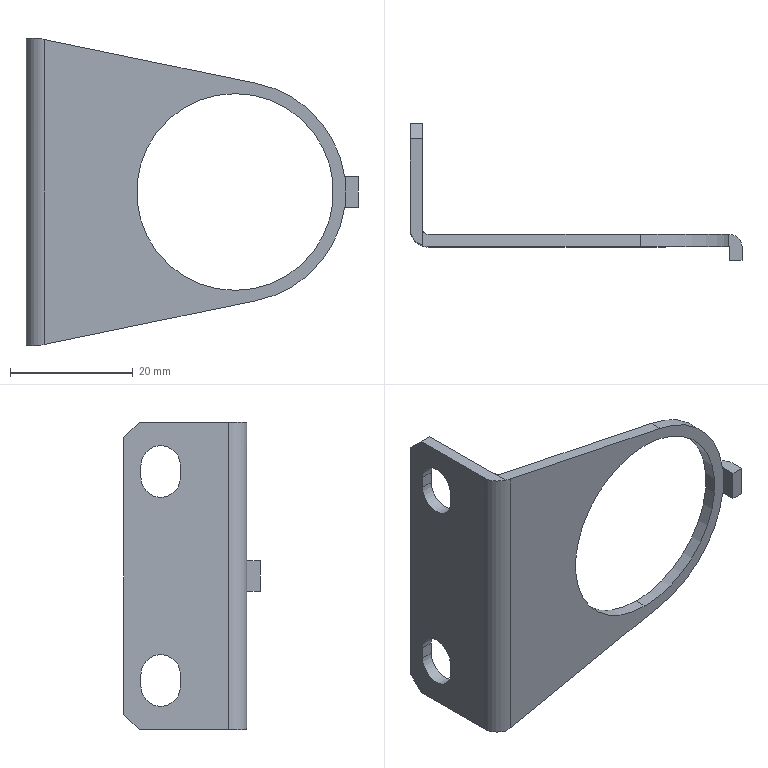Part | SolidWorks | features BaseBody 1 | 1 solid | 31 faces | box 54 x 22.2 x 50 mm | volume 3948 mm3 | plane 20 | cylinder 11 | commonest cylinder face diameters 6.4 x4 32 x2 36 x2 2 x1 4 x1 6 x1
STEP:
#1=CARTESIAN_POINT('',(0.,2.,16.));
#2=VERTEX_POINT('',#1);
#3=CARTESIAN_POINT('',(0.,2.,-16.));
#4=VERTEX_POINT('',#3);
#5=CARTESIAN_POINT('',(0.,2.,0.));
#6=DIRECTION('',(0.,1.,0.));
#7=DIRECTION('',(0.,0.,1.));
#8=AXIS2_PLACEMENT_3D('',#5,#6,#7);
#9=CIRCLE('',#8,16.);
#10=EDGE_CURVE('',#2,#4,#9,.T.);
#11=ORIENTED_EDGE('',*,*,#10,.T.);
#12=CARTESIAN_POINT('',(0.,0.,-16.));
#13=VERTEX_POINT('',#12);
#14=CARTESIAN_POINT('',(0.,2.,-16.));
#15=DIRECTION('',(0.,-1.,0.));
#16=VECTOR('',#15,1000.);
#17=LINE('',#14,#16);
#18=EDGE_CURVE('',#4,#13,#17,.T.);
#19=ORIENTED_EDGE('',*,*,#18,.T.);
#20=CARTESIAN_POINT('',(0.,0.,16.));
#21=VERTEX_POINT('',#20);
#22=CARTESIAN_POINT('',(0.,0.,0.));
#23=DIRECTION('',(0.,1.,0.));
#24=DIRECTION('',(0.,0.,-1.));
#25=AXIS2_PLACEMENT_3D('',#22,#23,#24);
#26=CIRCLE('',#25,16.);
#27=EDGE_CURVE('',#21,#13,#26,.T.);
#28=ORIENTED_EDGE('',*,*,#27,.F.);
#29=CARTESIAN_POINT('',(0.,2.,16.));
#30=DIRECTION('',(0.,-1.,0.));
#31=VECTOR('',#30,1000.);
#32=LINE('',#29,#31);
#33=EDGE_CURVE('',#2,#21,#32,.T.);
#34=ORIENTED_EDGE('',*,*,#33,.F.);
#35=EDGE_LOOP('',(#11,#19,#28,#34));
#36=FACE_OUTER_BOUND('',#35,.T.);
#37=CARTESIAN_POINT('',(0.,2.,0.));
#38=DIRECTION('',(0.,-1.,0.));
#39=DIRECTION('',(0.,0.,1.));
#40=AXIS2_PLACEMENT_3D('',#37,#38,#39);
#41=CYLINDRICAL_SURFACE('',#40,16.);
#42=ADVANCED_FACE('',(#36),#41,.F.);
#43=CARTESIAN_POINT('',(-34.,20.,22.5));
#44=VERTEX_POINT('',#43);
#45=CARTESIAN_POINT('',(-34.,20.,-22.5));
#46=VERTEX_POINT('',#45);
#47=CARTESIAN_POINT('',(-34.,20.,-22.5));
#48=DIRECTION('',(0.,0.,-1.));
#49=VECTOR('',#48,1000.);
#50=LINE('',#47,#49);
#51=EDGE_CURVE('',#44,#46,#50,.T.);
#52=ORIENTED_EDGE('',*,*,#51,.F.);
#53=CARTESIAN_POINT('',(-32.,20.,22.5));
#54=VERTEX_POINT('',#53);
#55=CARTESIAN_POINT('',(-34.,20.,22.5));
#56=DIRECTION('',(1.,0.,0.));
#57=VECTOR('',#56,1000.);
#58=LINE('',#55,#57);
#59=EDGE_CURVE('',#44,#54,#58,.T.);
#60=ORIENTED_EDGE('',*,*,#59,.T.);
#61=CARTESIAN_POINT('',(-32.,20.,-22.5));
#62=VERTEX_POINT('',#61);
#63=CARTESIAN_POINT('',(-32.,20.,22.5));
#64=DIRECTION('',(0.,0.,-1.));
#65=VECTOR('',#64,1000.);
#66=LINE('',#63,#65);
#67=EDGE_CURVE('',#54,#62,#66,.T.);
#68=ORIENTED_EDGE('',*,*,#67,.T.);
#69=CARTESIAN_POINT('',(-32.,20.,-22.5));
#70=DIRECTION('',(1.,0.,0.));
#71=VECTOR('',#70,1000.);
#72=LINE('',#69,#71);
#73=EDGE_CURVE('',#46,#62,#72,.T.);
#74=ORIENTED_EDGE('',*,*,#73,.F.);
#75=EDGE_LOOP('',(#52,#60,#68,#74));
#76=FACE_OUTER_BOUND('',#75,.T.);
#77=CARTESIAN_POINT('',(-34.,20.,22.5));
#78=DIRECTION('',(0.,1.,0.));
#79=DIRECTION('',(1.,0.,0.));
#80=AXIS2_PLACEMENT_3D('',#77,#78,#79);
#81=PLANE('',#80);
#82=ADVANCED_FACE('',(#76),#81,.T.);
#83=CARTESIAN_POINT('',(-34.,17.5,-25.));
#84=VERTEX_POINT('',#83);
#85=CARTESIAN_POINT('',(-34.,3.,-25.));
#86=VERTEX_POINT('',#85);
#87=CARTESIAN_POINT('',(-34.,17.5,-25.));
#88=DIRECTION('',(0.,-1.,0.));
#89=VECTOR('',#88,1000.);
#90=LINE('',#87,#89);
#91=EDGE_CURVE('',#84,#86,#90,.T.);
#92=ORIENTED_EDGE('',*,*,#91,.T.);
#93=CARTESIAN_POINT('',(-34.,3.,25.));
#94=VERTEX_POINT('',#93);
#95=CARTESIAN_POINT('',(-34.,3.,-25.));
#96=DIRECTION('',(0.,0.,-1.));
#97=VECTOR('',#96,1000.);
#98=LINE('',#95,#97);
#99=EDGE_CURVE('',#94,#86,#98,.T.);
#100=ORIENTED_EDGE('',*,*,#99,.F.);
#101=CARTESIAN_POINT('',(-34.,17.5,25.));
#102=VERTEX_POINT('',#101);
#103=CARTESIAN_POINT('',(-34.,3.,25.));
#104=DIRECTION('',(0.,-1.,0.));
#105=VECTOR('',#104,1000.);
#106=LINE('',#103,#105);
#107=EDGE_CURVE('',#102,#94,#106,.T.);
#108=ORIENTED_EDGE('',*,*,#107,.F.);
#109=CARTESIAN_POINT('',(-34.,17.5,25.));
#110=DIRECTION('',(0.,0.7071,-0.7071));
#111=VECTOR('',#110,1000.);
#112=LINE('',#109,#111);
#113=EDGE_CURVE('',#102,#44,#112,.T.);
#114=ORIENTED_EDGE('',*,*,#113,.T.);
#115=ORIENTED_EDGE('',*,*,#51,.T.);
#116=CARTESIAN_POINT('',(-34.,20.,-22.5));
#117=DIRECTION('',(0.,-0.7071,-0.7071));
#118=VECTOR('',#117,1000.);
#119=LINE('',#116,#118);
#120=EDGE_CURVE('',#46,#84,#119,.T.);
#121=ORIENTED_EDGE('',*,*,#120,.T.);
#122=EDGE_LOOP('',(#92,#100,#108,#114,#115,#121));
#123=FACE_OUTER_BOUND('',#122,.T.);
#124=CARTESIAN_POINT('',(-34.,10.8,16.));
#125=VERTEX_POINT('',#124);
#126=CARTESIAN_POINT('',(-34.,17.2,16.));
#127=VERTEX_POINT('',#126);
#128=CARTESIAN_POINT('',(-34.,14.,16.));
#129=DIRECTION('',(1.,0.,0.));
#130=DIRECTION('',(0.,-1.,0.));
#131=AXIS2_PLACEMENT_3D('',#128,#129,#130);
#132=CIRCLE('',#131,3.2);
#133=EDGE_CURVE('',#125,#127,#132,.T.);
#134=ORIENTED_EDGE('',*,*,#133,.T.);
#135=CARTESIAN_POINT('',(-34.,17.2,18.));
#136=VERTEX_POINT('',#135);
#137=CARTESIAN_POINT('',(-34.,17.2,16.));
#138=DIRECTION('',(0.,0.,1.));
#139=VECTOR('',#138,1000.);
#140=LINE('',#137,#139);
#141=EDGE_CURVE('',#127,#136,#140,.T.);
#142=ORIENTED_EDGE('',*,*,#141,.T.);
#143=CARTESIAN_POINT('',(-34.,10.8,18.));
#144=VERTEX_POINT('',#143);
#145=CARTESIAN_POINT('',(-34.,14.,18.));
#146=DIRECTION('',(1.,0.,0.));
#147=DIRECTION('',(0.,1.,0.));
#148=AXIS2_PLACEMENT_3D('',#145,#146,#147);
#149=CIRCLE('',#148,3.2);
#150=EDGE_CURVE('',#136,#144,#149,.T.);
#151=ORIENTED_EDGE('',*,*,#150,.T.);
#152=CARTESIAN_POINT('',(-34.,10.8,18.));
#153=DIRECTION('',(0.,0.,-1.));
#154=VECTOR('',#153,1000.);
#155=LINE('',#152,#154);
#156=EDGE_CURVE('',#144,#125,#155,.T.);
#157=ORIENTED_EDGE('',*,*,#156,.T.);
#158=EDGE_LOOP('',(#134,#142,#151,#157));
#159=FACE_BOUND('',#158,.T.);
#160=CARTESIAN_POINT('',(-34.,10.8,-18.));
#161=VERTEX_POINT('',#160);
#162=CARTESIAN_POINT('',(-34.,17.2,-18.));
#163=VERTEX_POINT('',#162);
#164=CARTESIAN_POINT('',(-34.,14.,-18.));
#165=DIRECTION('',(1.,0.,0.));
#166=DIRECTION('',(0.,-1.,0.));
#167=AXIS2_PLACEMENT_3D('',#164,#165,#166);
#168=CIRCLE('',#167,3.2);
#169=EDGE_CURVE('',#161,#163,#168,.T.);
#170=ORIENTED_EDGE('',*,*,#169,.T.);
#171=CARTESIAN_POINT('',(-34.,17.2,-16.));
#172=VERTEX_POINT('',#171);
#173=CARTESIAN_POINT('',(-34.,17.2,-18.));
#174=DIRECTION('',(0.,0.,1.));
#175=VECTOR('',#174,1000.);
#176=LINE('',#173,#175);
#177=EDGE_CURVE('',#163,#172,#176,.T.);
#178=ORIENTED_EDGE('',*,*,#177,.T.);
#179=CARTESIAN_POINT('',(-34.,10.8,-16.));
#180=VERTEX_POINT('',#179);
#181=CARTESIAN_POINT('',(-34.,14.,-16.));
#182=DIRECTION('',(1.,0.,0.));
#183=DIRECTION('',(0.,1.,0.));
#184=AXIS2_PLACEMENT_3D('',#181,#182,#183);
#185=CIRCLE('',#184,3.2);
#186=EDGE_CURVE('',#172,#180,#185,.T.);
#187=ORIENTED_EDGE('',*,*,#186,.T.);
#188=CARTESIAN_POINT('',(-34.,10.8,-16.));
#189=DIRECTION('',(0.,0.,-1.));
#190=VECTOR('',#189,1000.);
#191=LINE('',#188,#190);
#192=EDGE_CURVE('',#180,#161,#191,.T.);
#193=ORIENTED_EDGE('',*,*,#192,.T.);
#194=EDGE_LOOP('',(#170,#178,#187,#193));
#195=FACE_BOUND('',#194,.T.);
#196=CARTESIAN_POINT('',(-34.,3.,25.));
#197=DIRECTION('',(-1.,0.,0.));
#198=DIRECTION('',(0.,1.,0.));
#199=AXIS2_PLACEMENT_3D('',#196,#197,#198);
#200=PLANE('',#199);
#201=ADVANCED_FACE('',(#123,#159,#195),#200,.T.);
#202=CARTESIAN_POINT('',(-32.,0.1716,-25.));
#203=VERTEX_POINT('',#202);
#204=CARTESIAN_POINT('',(-31.,3.,-25.));
#205=DIRECTION('',(0.,0.,1.));
#206=DIRECTION('',(-1.,0.,0.));
#207=AXIS2_PLACEMENT_3D('',#204,#205,#206);
#208=CIRCLE('',#207,3.);
#209=EDGE_CURVE('',#86,#203,#208,.T.);
#210=ORIENTED_EDGE('',*,*,#209,.T.);
#211=CARTESIAN_POINT('',(-31.,0.,-24.793));
#212=VERTEX_POINT('',#211);
#213=CARTESIAN_POINT('',(-32.,0.1716,-25.));
#214=CARTESIAN_POINT('',(-31.679,0.05802,-24.934));
#215=CARTESIAN_POINT('',(-31.341,0.,-24.864));
#216=CARTESIAN_POINT('',(-31.,0.,-24.793));
#217=B_SPLINE_CURVE_WITH_KNOTS('',3,(#213,#214,#215,#216),.UNSPECIFIED.,.F.,.F.,(4,4),(0.,1.),.UNSPECIFIED.);
#218=EDGE_CURVE('',#203,#212,#217,.T.);
#219=ORIENTED_EDGE('',*,*,#218,.T.);
#220=CARTESIAN_POINT('',(-31.,0.,24.793));
#221=VERTEX_POINT('',#220);
#222=CARTESIAN_POINT('',(-31.,0.,-24.793));
#223=DIRECTION('',(0.,0.,-1.));
#224=VECTOR('',#223,1000.);
#225=LINE('',#222,#224);
#226=EDGE_CURVE('',#221,#212,#225,.T.);
#227=ORIENTED_EDGE('',*,*,#226,.F.);
#228=CARTESIAN_POINT('',(-32.,0.1716,25.));
#229=VERTEX_POINT('',#228);
#230=CARTESIAN_POINT('',(-31.,0.,24.793));
#231=CARTESIAN_POINT('',(-31.341,0.,24.864));
#232=CARTESIAN_POINT('',(-31.679,0.05802,24.934));
#233=CARTESIAN_POINT('',(-32.,0.1716,25.));
#234=B_SPLINE_CURVE_WITH_KNOTS('',3,(#230,#231,#232,#233),.UNSPECIFIED.,.F.,.F.,(4,4),(0.,1.),.UNSPECIFIED.);
#235=EDGE_CURVE('',#221,#229,#234,.T.);
#236=ORIENTED_EDGE('',*,*,#235,.T.);
#237=CARTESIAN_POINT('',(-31.,3.,25.));
#238=DIRECTION('',(0.,0.,1.));
#239=DIRECTION('',(-0.3333,-0.9428,0.));
#240=AXIS2_PLACEMENT_3D('',#237,#238,#239);
#241=CIRCLE('',#240,3.);
#242=EDGE_CURVE('',#94,#229,#241,.T.);
#243=ORIENTED_EDGE('',*,*,#242,.F.);
#244=ORIENTED_EDGE('',*,*,#99,.T.);
#245=EDGE_LOOP('',(#210,#219,#227,#236,#243,#244));
#246=FACE_OUTER_BOUND('',#245,.T.);
#247=CARTESIAN_POINT('',(-31.,3.,25.));
#248=DIRECTION('',(0.,0.,-1.));
#249=DIRECTION('',(0.,-1.,0.));
#250=AXIS2_PLACEMENT_3D('',#247,#248,#249);
#251=CYLINDRICAL_SURFACE('',#250,3.);
#252=ADVANCED_FACE('',(#246),#251,.T.);
#253=ORIENTED_EDGE('',*,*,#226,.T.);
#254=CARTESIAN_POINT('',(3.459,0.,-17.664));
#255=VERTEX_POINT('',#254);
#256=CARTESIAN_POINT('',(-31.,0.,-24.793));
#257=DIRECTION('',(0.9793,0.,0.2026));
#258=VECTOR('',#257,1000.);
#259=LINE('',#256,#258);
#260=EDGE_CURVE('',#212,#255,#259,.T.);
#261=ORIENTED_EDGE('',*,*,#260,.T.);
#262=CARTESIAN_POINT('',(17.826,0.,-2.5));
#263=VERTEX_POINT('',#262);
#264=CARTESIAN_POINT('',(0.,0.,0.));
#265=DIRECTION('',(0.,-1.,0.));
#266=DIRECTION('',(0.1922,0.,-0.9814));
#267=AXIS2_PLACEMENT_3D('',#264,#265,#266);
#268=CIRCLE('',#267,18.);
#269=EDGE_CURVE('',#255,#263,#268,.T.);
#270=ORIENTED_EDGE('',*,*,#269,.T.);
#271=CARTESIAN_POINT('',(18.,0.,-2.5));
#272=VERTEX_POINT('',#271);
#273=CARTESIAN_POINT('',(17.826,0.,-2.5));
#274=DIRECTION('',(1.,0.,0.));
#275=VECTOR('',#274,1000.);
#276=LINE('',#273,#275);
#277=EDGE_CURVE('',#263,#272,#276,.T.);
#278=ORIENTED_EDGE('',*,*,#277,.T.);
#279=CARTESIAN_POINT('',(18.,0.,2.5));
#280=VERTEX_POINT('',#279);
#281=CARTESIAN_POINT('',(18.,0.,-2.5));
#282=DIRECTION('',(0.,0.,-1.));
#283=VECTOR('',#282,1000.);
#284=LINE('',#281,#283);
#285=EDGE_CURVE('',#280,#272,#284,.T.);
#286=ORIENTED_EDGE('',*,*,#285,.F.);
#287=CARTESIAN_POINT('',(17.826,0.,2.5));
#288=VERTEX_POINT('',#287);
#289=CARTESIAN_POINT('',(18.,0.,2.5));
#290=DIRECTION('',(-1.,0.,0.));
#291=VECTOR('',#290,1000.);
#292=LINE('',#289,#291);
#293=EDGE_CURVE('',#280,#288,#292,.T.);
#294=ORIENTED_EDGE('',*,*,#293,.T.);
#295=CARTESIAN_POINT('',(3.459,0.,17.664));
#296=VERTEX_POINT('',#295);
#297=CARTESIAN_POINT('',(0.,0.,0.));
#298=DIRECTION('',(0.,-1.,0.));
#299=DIRECTION('',(0.9903,0.,0.1389));
#300=AXIS2_PLACEMENT_3D('',#297,#298,#299);
#301=CIRCLE('',#300,18.);
#302=EDGE_CURVE('',#288,#296,#301,.T.);
#303=ORIENTED_EDGE('',*,*,#302,.T.);
#304=CARTESIAN_POINT('',(3.459,0.,17.664));
#305=DIRECTION('',(-0.9793,0.,0.2026));
#306=VECTOR('',#305,1000.);
#307=LINE('',#304,#306);
#308=EDGE_CURVE('',#296,#221,#307,.T.);
#309=ORIENTED_EDGE('',*,*,#308,.T.);
#310=EDGE_LOOP('',(#253,#261,#270,#278,#286,#294,#303,#309));
#311=FACE_OUTER_BOUND('',#310,.T.);
#312=ORIENTED_EDGE('',*,*,#27,.T.);
#313=CARTESIAN_POINT('',(0.,0.,0.));
#314=DIRECTION('',(0.,1.,0.));
#315=DIRECTION('',(0.,0.,-1.));
#316=AXIS2_PLACEMENT_3D('',#313,#314,#315);
#317=CIRCLE('',#316,16.);
#318=EDGE_CURVE('',#13,#21,#317,.T.);
#319=ORIENTED_EDGE('',*,*,#318,.T.);
#320=EDGE_LOOP('',(#312,#319));
#321=FACE_BOUND('',#320,.T.);
#322=CARTESIAN_POINT('',(-31.,0.,-24.793));
#323=DIRECTION('',(0.,-1.,0.));
#324=DIRECTION('',(1.,0.,0.));
#325=AXIS2_PLACEMENT_3D('',#322,#323,#324);
#326=PLANE('',#325);
#327=ADVANCED_FACE('',(#311,#321),#326,.T.);
#328=ORIENTED_EDGE('',*,*,#285,.T.);
#329=CARTESIAN_POINT('',(18.,-2.2,-2.5));
#330=VERTEX_POINT('',#329);
#331=CARTESIAN_POINT('',(18.,0.,-2.5));
#332=DIRECTION('',(0.,-1.,0.));
#333=VECTOR('',#332,1000.);
#334=LINE('',#331,#333);
#335=EDGE_CURVE('',#272,#330,#334,.T.);
#336=ORIENTED_EDGE('',*,*,#335,.T.);
#337=CARTESIAN_POINT('',(18.,-2.2,2.5));
#338=VERTEX_POINT('',#337);
#339=CARTESIAN_POINT('',(18.,-2.2,-2.5));
#340=DIRECTION('',(0.,0.,-1.));
#341=VECTOR('',#340,1000.);
#342=LINE('',#339,#341);
#343=EDGE_CURVE('',#338,#330,#342,.T.);
#344=ORIENTED_EDGE('',*,*,#343,.F.);
#345=CARTESIAN_POINT('',(18.,-2.2,2.5));
#346=DIRECTION('',(0.,1.,0.));
#347=VECTOR('',#346,1000.);
#348=LINE('',#345,#347);
#349=EDGE_CURVE('',#338,#280,#348,.T.);
#350=ORIENTED_EDGE('',*,*,#349,.T.);
#351=EDGE_LOOP('',(#328,#336,#344,#350));
#352=FACE_OUTER_BOUND('',#351,.T.);
#353=CARTESIAN_POINT('',(18.,-2.2,2.5));
#354=DIRECTION('',(-1.,0.,0.));
#355=DIRECTION('',(0.,1.,0.));
#356=AXIS2_PLACEMENT_3D('',#353,#354,#355);
#357=PLANE('',#356);
#358=ADVANCED_FACE('',(#352),#357,.T.);
#359=ORIENTED_EDGE('',*,*,#343,.T.);
#360=CARTESIAN_POINT('',(20.,-2.2,-2.5));
#361=VERTEX_POINT('',#360);
#362=CARTESIAN_POINT('',(18.,-2.2,-2.5));
#363=DIRECTION('',(1.,0.,0.));
#364=VECTOR('',#363,1000.);
#365=LINE('',#362,#364);
#366=EDGE_CURVE('',#330,#361,#365,.T.);
#367=ORIENTED_EDGE('',*,*,#366,.T.);
#368=CARTESIAN_POINT('',(20.,-2.2,2.5));
#369=VERTEX_POINT('',#368);
#370=CARTESIAN_POINT('',(20.,-2.2,-2.5));
#371=DIRECTION('',(0.,0.,-1.));
#372=VECTOR('',#371,1000.);
#373=LINE('',#370,#372);
#374=EDGE_CURVE('',#369,#361,#373,.T.);
#375=ORIENTED_EDGE('',*,*,#374,.F.);
#376=CARTESIAN_POINT('',(20.,-2.2,2.5));
#377=DIRECTION('',(-1.,0.,0.));
#378=VECTOR('',#377,1000.);
#379=LINE('',#376,#378);
#380=EDGE_CURVE('',#369,#338,#379,.T.);
#381=ORIENTED_EDGE('',*,*,#380,.T.);
#382=EDGE_LOOP('',(#359,#367,#375,#381));
#383=FACE_OUTER_BOUND('',#382,.T.);
#384=CARTESIAN_POINT('',(18.,-2.2,-2.5));
#385=DIRECTION('',(0.,-1.,0.));
#386=DIRECTION('',(1.,0.,0.));
#387=AXIS2_PLACEMENT_3D('',#384,#385,#386);
#388=PLANE('',#387);
#389=ADVANCED_FACE('',(#383),#388,.T.);
#390=ORIENTED_EDGE('',*,*,#374,.T.);
#391=CARTESIAN_POINT('',(20.,0.,-2.5));
#392=VERTEX_POINT('',#391);
#393=CARTESIAN_POINT('',(20.,-2.2,-2.5));
#394=DIRECTION('',(0.,1.,0.));
#395=VECTOR('',#394,1000.);
#396=LINE('',#393,#395);
#397=EDGE_CURVE('',#361,#392,#396,.T.);
#398=ORIENTED_EDGE('',*,*,#397,.T.);
#399=CARTESIAN_POINT('',(20.,0.,2.5));
#400=VERTEX_POINT('',#399);
#401=CARTESIAN_POINT('',(20.,0.,-2.5));
#402=DIRECTION('',(0.,0.,-1.));
#403=VECTOR('',#402,1000.);
#404=LINE('',#401,#403);
#405=EDGE_CURVE('',#400,#392,#404,.T.);
#406=ORIENTED_EDGE('',*,*,#405,.F.);
#407=CARTESIAN_POINT('',(20.,0.,2.5));
#408=DIRECTION('',(0.,-1.,0.));
#409=VECTOR('',#408,1000.);
#410=LINE('',#407,#409);
#411=EDGE_CURVE('',#400,#369,#410,.T.);
#412=ORIENTED_EDGE('',*,*,#411,.T.);
#413=EDGE_LOOP('',(#390,#398,#406,#412));
#414=FACE_OUTER_BOUND('',#413,.T.);
#415=CARTESIAN_POINT('',(20.,-2.2,-2.5));
#416=DIRECTION('',(1.,0.,0.));
#417=DIRECTION('',(0.,1.,0.));
#418=AXIS2_PLACEMENT_3D('',#415,#416,#417);
#419=PLANE('',#418);
#420=ADVANCED_FACE('',(#414),#419,.T.);
#421=ORIENTED_EDGE('',*,*,#405,.T.);
#422=CARTESIAN_POINT('',(18.,2.,-2.5));
#423=VERTEX_POINT('',#422);
#424=CARTESIAN_POINT('',(18.,0.,-2.5));
#425=DIRECTION('',(0.,0.,1.));
#426=DIRECTION('',(1.,0.,0.));
#427=AXIS2_PLACEMENT_3D('',#424,#425,#426);
#428=CIRCLE('',#427,2.);
#429=EDGE_CURVE('',#392,#423,#428,.T.);
#430=ORIENTED_EDGE('',*,*,#429,.T.);
#431=CARTESIAN_POINT('',(18.,2.,2.5));
#432=VERTEX_POINT('',#431);
#433=CARTESIAN_POINT('',(18.,2.,-2.5));
#434=DIRECTION('',(0.,0.,-1.));
#435=VECTOR('',#434,1000.);
#436=LINE('',#433,#435);
#437=EDGE_CURVE('',#432,#423,#436,.T.);
#438=ORIENTED_EDGE('',*,*,#437,.F.);
#439=CARTESIAN_POINT('',(18.,0.,2.5));
#440=DIRECTION('',(0.,0.,-1.));
#441=DIRECTION('',(0.,1.,0.));
#442=AXIS2_PLACEMENT_3D('',#439,#440,#441);
#443=CIRCLE('',#442,2.);
#444=EDGE_CURVE('',#432,#400,#443,.T.);
#445=ORIENTED_EDGE('',*,*,#444,.T.);
#446=EDGE_LOOP('',(#421,#430,#438,#445));
#447=FACE_OUTER_BOUND('',#446,.T.);
#448=CARTESIAN_POINT('',(18.,0.,25.));
#449=DIRECTION('',(0.,0.,-1.));
#450=DIRECTION('',(0.,1.,0.));
#451=AXIS2_PLACEMENT_3D('',#448,#449,#450);
#452=CYLINDRICAL_SURFACE('',#451,2.);
#453=ADVANCED_FACE('',(#447),#452,.T.);
#454=CARTESIAN_POINT('',(17.826,2.,-2.5));
#455=VERTEX_POINT('',#454);
#456=CARTESIAN_POINT('',(3.459,2.,-17.664));
#457=VERTEX_POINT('',#456);
#458=CARTESIAN_POINT('',(0.,2.,0.));
#459=DIRECTION('',(0.,1.,0.));
#460=DIRECTION('',(0.9903,0.,-0.1389));
#461=AXIS2_PLACEMENT_3D('',#458,#459,#460);
#462=CIRCLE('',#461,18.);
#463=EDGE_CURVE('',#455,#457,#462,.T.);
#464=ORIENTED_EDGE('',*,*,#463,.T.);
#465=CARTESIAN_POINT('',(-31.,2.,-24.793));
#466=VERTEX_POINT('',#465);
#467=CARTESIAN_POINT('',(3.459,2.,-17.664));
#468=DIRECTION('',(-0.9793,0.,-0.2026));
#469=VECTOR('',#468,1000.);
#470=LINE('',#467,#469);
#471=EDGE_CURVE('',#457,#466,#470,.T.);
#472=ORIENTED_EDGE('',*,*,#471,.T.);
#473=CARTESIAN_POINT('',(-31.,2.,24.793));
#474=VERTEX_POINT('',#473);
#475=CARTESIAN_POINT('',(-31.,2.,-24.793));
#476=DIRECTION('',(0.,0.,-1.));
#477=VECTOR('',#476,1000.);
#478=LINE('',#475,#477);
#479=EDGE_CURVE('',#474,#466,#478,.T.);
#480=ORIENTED_EDGE('',*,*,#479,.F.);
#481=CARTESIAN_POINT('',(3.459,2.,17.664));
#482=VERTEX_POINT('',#481);
#483=CARTESIAN_POINT('',(-31.,2.,24.793));
#484=DIRECTION('',(0.9793,0.,-0.2026));
#485=VECTOR('',#484,1000.);
#486=LINE('',#483,#485);
#487=EDGE_CURVE('',#474,#482,#486,.T.);
#488=ORIENTED_EDGE('',*,*,#487,.T.);
#489=CARTESIAN_POINT('',(17.826,2.,2.5));
#490=VERTEX_POINT('',#489);
#491=CARTESIAN_POINT('',(0.,2.,0.));
#492=DIRECTION('',(0.,1.,0.));
#493=DIRECTION('',(0.1922,0.,0.9814));
#494=AXIS2_PLACEMENT_3D('',#491,#492,#493);
#495=CIRCLE('',#494,18.);
#496=EDGE_CURVE('',#482,#490,#495,.T.);
#497=ORIENTED_EDGE('',*,*,#496,.T.);
#498=CARTESIAN_POINT('',(17.826,2.,2.5));
#499=DIRECTION('',(1.,0.,0.));
#500=VECTOR('',#499,1000.);
#501=LINE('',#498,#500);
#502=EDGE_CURVE('',#490,#432,#501,.T.);
#503=ORIENTED_EDGE('',*,*,#502,.T.);
#504=ORIENTED_EDGE('',*,*,#437,.T.);
#505=CARTESIAN_POINT('',(18.,2.,-2.5));
#506=DIRECTION('',(-1.,0.,0.));
#507=VECTOR('',#506,1000.);
#508=LINE('',#505,#507);
#509=EDGE_CURVE('',#423,#455,#508,.T.);
#510=ORIENTED_EDGE('',*,*,#509,.T.);
#511=EDGE_LOOP('',(#464,#472,#480,#488,#497,#503,#504,#510));
#512=FACE_OUTER_BOUND('',#511,.T.);
#513=ORIENTED_EDGE('',*,*,#10,.F.);
#514=CARTESIAN_POINT('',(0.,2.,0.));
#515=DIRECTION('',(0.,1.,0.));
#516=DIRECTION('',(0.,0.,1.));
#517=AXIS2_PLACEMENT_3D('',#514,#515,#516);
#518=CIRCLE('',#517,16.);
#519=EDGE_CURVE('',#4,#2,#518,.T.);
#520=ORIENTED_EDGE('',*,*,#519,.F.);
#521=EDGE_LOOP('',(#513,#520));
#522=FACE_BOUND('',#521,.T.);
#523=CARTESIAN_POINT('',(-31.,2.,24.793));
#524=DIRECTION('',(0.,1.,0.));
#525=DIRECTION('',(1.,0.,0.));
#526=AXIS2_PLACEMENT_3D('',#523,#524,#525);
#527=PLANE('',#526);
#528=ADVANCED_FACE('',(#512,#522),#527,.T.);
#529=CARTESIAN_POINT('',(-32.,3.,-25.));
#530=VERTEX_POINT('',#529);
#531=CARTESIAN_POINT('',(-32.,3.,-25.));
#532=CARTESIAN_POINT('',(-32.,2.775,-25.));
#533=CARTESIAN_POINT('',(-31.925,2.553,-24.984));
#534=CARTESIAN_POINT('',(-31.706,2.283,-24.939));
#535=CARTESIAN_POINT('',(-31.62,2.204,-24.921));
#536=CARTESIAN_POINT('',(-31.45,2.105,-24.886));
#537=CARTESIAN_POINT('',(-31.389,2.075,-24.874));
#538=CARTESIAN_POINT('',(-31.272,2.037,-24.849));
#539=CARTESIAN_POINT('',(-31.228,2.025,-24.84));
#540=CARTESIAN_POINT('',(-31.154,2.011,-24.825));
#541=CARTESIAN_POINT('',(-31.129,2.008,-24.82));
#542=CARTESIAN_POINT('',(-31.071,2.002,-24.808));
#543=CARTESIAN_POINT('',(-31.035,2.,-24.8));
#544=CARTESIAN_POINT('',(-31.,2.,-24.793));
#545=B_SPLINE_CURVE_WITH_KNOTS('',3,(#531,#532,#533,#534,#535,#536,#537,#538,#539,#540,#541,#542,#543,#544),.UNSPECIFIED.,.F.,.F.,(4,2,2,2,2,2,4),(0.,0.5,0.75,0.875,0.9375,0.9687,1.),.UNSPECIFIED.);
#546=EDGE_CURVE('',#530,#466,#545,.T.);
#547=ORIENTED_EDGE('',*,*,#546,.F.);
#548=CARTESIAN_POINT('',(-32.,3.,25.));
#549=VERTEX_POINT('',#548);
#550=CARTESIAN_POINT('',(-32.,3.,-25.));
#551=DIRECTION('',(0.,0.,-1.));
#552=VECTOR('',#551,1000.);
#553=LINE('',#550,#552);
#554=EDGE_CURVE('',#549,#530,#553,.T.);
#555=ORIENTED_EDGE('',*,*,#554,.F.);
#556=CARTESIAN_POINT('',(-31.,2.,24.793));
#557=CARTESIAN_POINT('',(-31.04,2.,24.801));
#558=CARTESIAN_POINT('',(-31.072,2.002,24.808));
#559=CARTESIAN_POINT('',(-31.131,2.008,24.82));
#560=CARTESIAN_POINT('',(-31.159,2.012,24.826));
#561=CARTESIAN_POINT('',(-31.232,2.026,24.841));
#562=CARTESIAN_POINT('',(-31.273,2.037,24.85));
#563=CARTESIAN_POINT('',(-31.388,2.074,24.873));
#564=CARTESIAN_POINT('',(-31.449,2.104,24.886));
#565=CARTESIAN_POINT('',(-31.618,2.202,24.921));
#566=CARTESIAN_POINT('',(-31.705,2.282,24.939));
#567=CARTESIAN_POINT('',(-31.924,2.553,24.984));
#568=CARTESIAN_POINT('',(-32.,2.774,25.));
#569=CARTESIAN_POINT('',(-32.,3.,25.));
#570=B_SPLINE_CURVE_WITH_KNOTS('',3,(#556,#557,#558,#559,#560,#561,#562,#563,#564,#565,#566,#567,#568,#569),.UNSPECIFIED.,.F.,.F.,(4,2,2,2,2,2,4),(0.,0.03125,0.0625,0.125,0.25,0.5,1.),.UNSPECIFIED.);
#571=EDGE_CURVE('',#474,#549,#570,.T.);
#572=ORIENTED_EDGE('',*,*,#571,.F.);
#573=ORIENTED_EDGE('',*,*,#479,.T.);
#574=EDGE_LOOP('',(#547,#555,#572,#573));
#575=FACE_OUTER_BOUND('',#574,.T.);
#576=CARTESIAN_POINT('',(-31.,3.,25.));
#577=DIRECTION('',(0.,0.,-1.));
#578=DIRECTION('',(0.,-1.,0.));
#579=AXIS2_PLACEMENT_3D('',#576,#577,#578);
#580=CYLINDRICAL_SURFACE('',#579,1.);
#581=ADVANCED_FACE('',(#575),#580,.F.);
#582=ORIENTED_EDGE('',*,*,#67,.F.);
#583=CARTESIAN_POINT('',(-32.,17.5,25.));
#584=VERTEX_POINT('',#583);
#585=CARTESIAN_POINT('',(-32.,20.,22.5));
#586=DIRECTION('',(0.,-0.7071,0.7071));
#587=VECTOR('',#586,1000.);
#588=LINE('',#585,#587);
#589=EDGE_CURVE('',#54,#584,#588,.T.);
#590=ORIENTED_EDGE('',*,*,#589,.T.);
#591=CARTESIAN_POINT('',(-32.,17.5,25.));
#592=DIRECTION('',(0.,1.,0.));
#593=VECTOR('',#592,1000.);
#594=LINE('',#591,#593);
#595=EDGE_CURVE('',#549,#584,#594,.T.);
#596=ORIENTED_EDGE('',*,*,#595,.F.);
#597=ORIENTED_EDGE('',*,*,#554,.T.);
#598=CARTESIAN_POINT('',(-32.,17.5,-25.));
#599=VERTEX_POINT('',#598);
#600=CARTESIAN_POINT('',(-32.,3.,-25.));
#601=DIRECTION('',(0.,1.,0.));
#602=VECTOR('',#601,1000.);
#603=LINE('',#600,#602);
#604=EDGE_CURVE('',#530,#599,#603,.T.);
#605=ORIENTED_EDGE('',*,*,#604,.T.);
#606=CARTESIAN_POINT('',(-32.,17.5,-25.));
#607=DIRECTION('',(0.,0.7071,0.7071));
#608=VECTOR('',#607,1000.);
#609=LINE('',#606,#608);
#610=EDGE_CURVE('',#599,#62,#609,.T.);
#611=ORIENTED_EDGE('',*,*,#610,.T.);
#612=EDGE_LOOP('',(#582,#590,#596,#597,#605,#611));
#613=FACE_OUTER_BOUND('',#612,.T.);
#614=CARTESIAN_POINT('',(-32.,10.8,18.));
#615=VERTEX_POINT('',#614);
#616=CARTESIAN_POINT('',(-32.,17.2,18.));
#617=VERTEX_POINT('',#616);
#618=CARTESIAN_POINT('',(-32.,14.,18.));
#619=DIRECTION('',(-1.,0.,0.));
#620=DIRECTION('',(0.,-1.,0.));
#621=AXIS2_PLACEMENT_3D('',#618,#619,#620);
#622=CIRCLE('',#621,3.2);
#623=EDGE_CURVE('',#615,#617,#622,.T.);
#624=ORIENTED_EDGE('',*,*,#623,.T.);
#625=CARTESIAN_POINT('',(-32.,17.2,16.));
#626=VERTEX_POINT('',#625);
#627=CARTESIAN_POINT('',(-32.,17.2,18.));
#628=DIRECTION('',(0.,0.,-1.));
#629=VECTOR('',#628,1000.);
#630=LINE('',#627,#629);
#631=EDGE_CURVE('',#617,#626,#630,.T.);
#632=ORIENTED_EDGE('',*,*,#631,.T.);
#633=CARTESIAN_POINT('',(-32.,10.8,16.));
#634=VERTEX_POINT('',#633);
#635=CARTESIAN_POINT('',(-32.,14.,16.));
#636=DIRECTION('',(-1.,0.,0.));
#637=DIRECTION('',(0.,1.,0.));
#638=AXIS2_PLACEMENT_3D('',#635,#636,#637);
#639=CIRCLE('',#638,3.2);
#640=EDGE_CURVE('',#626,#634,#639,.T.);
#641=ORIENTED_EDGE('',*,*,#640,.T.);
#642=CARTESIAN_POINT('',(-32.,10.8,16.));
#643=DIRECTION('',(0.,0.,1.));
#644=VECTOR('',#643,1000.);
#645=LINE('',#642,#644);
#646=EDGE_CURVE('',#634,#615,#645,.T.);
#647=ORIENTED_EDGE('',*,*,#646,.T.);
#648=EDGE_LOOP('',(#624,#632,#641,#647));
#649=FACE_BOUND('',#648,.T.);
#650=CARTESIAN_POINT('',(-32.,10.8,-16.));
#651=VERTEX_POINT('',#650);
#652=CARTESIAN_POINT('',(-32.,17.2,-16.));
#653=VERTEX_POINT('',#652);
#654=CARTESIAN_POINT('',(-32.,14.,-16.));
#655=DIRECTION('',(-1.,0.,0.));
#656=DIRECTION('',(0.,-1.,0.));
#657=AXIS2_PLACEMENT_3D('',#654,#655,#656);
#658=CIRCLE('',#657,3.2);
#659=EDGE_CURVE('',#651,#653,#658,.T.);
#660=ORIENTED_EDGE('',*,*,#659,.T.);
#661=CARTESIAN_POINT('',(-32.,17.2,-18.));
#662=VERTEX_POINT('',#661);
#663=CARTESIAN_POINT('',(-32.,17.2,-16.));
#664=DIRECTION('',(0.,0.,-1.));
#665=VECTOR('',#664,1000.);
#666=LINE('',#663,#665);
#667=EDGE_CURVE('',#653,#662,#666,.T.);
#668=ORIENTED_EDGE('',*,*,#667,.T.);
#669=CARTESIAN_POINT('',(-32.,10.8,-18.));
#670=VERTEX_POINT('',#669);
#671=CARTESIAN_POINT('',(-32.,14.,-18.));
#672=DIRECTION('',(-1.,0.,0.));
#673=DIRECTION('',(0.,1.,0.));
#674=AXIS2_PLACEMENT_3D('',#671,#672,#673);
#675=CIRCLE('',#674,3.2);
#676=EDGE_CURVE('',#662,#670,#675,.T.);
#677=ORIENTED_EDGE('',*,*,#676,.T.);
#678=CARTESIAN_POINT('',(-32.,10.8,-18.));
#679=DIRECTION('',(0.,0.,1.));
#680=VECTOR('',#679,1000.);
#681=LINE('',#678,#680);
#682=EDGE_CURVE('',#670,#651,#681,.T.);
#683=ORIENTED_EDGE('',*,*,#682,.T.);
#684=EDGE_LOOP('',(#660,#668,#677,#683));
#685=FACE_BOUND('',#684,.T.);
#686=CARTESIAN_POINT('',(-32.,3.,-25.));
#687=DIRECTION('',(1.,0.,0.));
#688=DIRECTION('',(0.,1.,0.));
#689=AXIS2_PLACEMENT_3D('',#686,#687,#688);
#690=PLANE('',#689);
#691=ADVANCED_FACE('',(#613,#649,#685),#690,.T.);
#692=ORIENTED_EDGE('',*,*,#107,.T.);
#693=ORIENTED_EDGE('',*,*,#242,.T.);
#694=CARTESIAN_POINT('',(-32.,0.1716,25.));
#695=DIRECTION('',(0.,-1.,0.));
#696=VECTOR('',#695,1000.);
#697=LINE('',#694,#696);
#698=EDGE_CURVE('',#549,#229,#697,.T.);
#699=ORIENTED_EDGE('',*,*,#698,.F.);
#700=ORIENTED_EDGE('',*,*,#595,.T.);
#701=CARTESIAN_POINT('',(-32.,17.5,25.));
#702=DIRECTION('',(1.,0.,0.));
#703=VECTOR('',#702,1000.);
#704=LINE('',#701,#703);
#705=EDGE_CURVE('',#102,#584,#704,.T.);
#706=ORIENTED_EDGE('',*,*,#705,.F.);
#707=EDGE_LOOP('',(#692,#693,#699,#700,#706));
#708=FACE_OUTER_BOUND('',#707,.T.);
#709=CARTESIAN_POINT('',(-34.,0.1716,25.));
#710=DIRECTION('',(0.,0.,1.));
#711=DIRECTION('',(1.,0.,0.));
#712=AXIS2_PLACEMENT_3D('',#709,#710,#711);
#713=PLANE('',#712);
#714=ADVANCED_FACE('',(#708),#713,.T.);
#715=CARTESIAN_POINT('',(-34.,17.5,-25.));
#716=DIRECTION('',(1.,0.,0.));
#717=VECTOR('',#716,1000.);
#718=LINE('',#715,#717);
#719=EDGE_CURVE('',#84,#599,#718,.T.);
#720=ORIENTED_EDGE('',*,*,#719,.T.);
#721=ORIENTED_EDGE('',*,*,#604,.F.);
#722=CARTESIAN_POINT('',(-32.,3.,-25.));
#723=DIRECTION('',(0.,-1.,0.));
#724=VECTOR('',#723,1000.);
#725=LINE('',#722,#724);
#726=EDGE_CURVE('',#530,#203,#725,.T.);
#727=ORIENTED_EDGE('',*,*,#726,.T.);
#728=ORIENTED_EDGE('',*,*,#209,.F.);
#729=ORIENTED_EDGE('',*,*,#91,.F.);
#730=EDGE_LOOP('',(#720,#721,#727,#728,#729));
#731=FACE_OUTER_BOUND('',#730,.T.);
#732=CARTESIAN_POINT('',(-34.,0.1716,-25.));
#733=DIRECTION('',(0.,0.,-1.));
#734=DIRECTION('',(0.,1.,0.));
#735=AXIS2_PLACEMENT_3D('',#732,#733,#734);
#736=PLANE('',#735);
#737=ADVANCED_FACE('',(#731),#736,.T.);
#738=ORIENTED_EDGE('',*,*,#719,.F.);
#739=ORIENTED_EDGE('',*,*,#120,.F.);
#740=ORIENTED_EDGE('',*,*,#73,.T.);
#741=ORIENTED_EDGE('',*,*,#610,.F.);
#742=EDGE_LOOP('',(#738,#739,#740,#741));
#743=FACE_OUTER_BOUND('',#742,.T.);
#744=CARTESIAN_POINT('',(-34.,20.,-22.5));
#745=DIRECTION('',(0.,0.7071,-0.7071));
#746=DIRECTION('',(1.,0.,0.));
#747=AXIS2_PLACEMENT_3D('',#744,#745,#746);
#748=PLANE('',#747);
#749=ADVANCED_FACE('',(#743),#748,.T.);
#750=ORIENTED_EDGE('',*,*,#59,.F.);
#751=ORIENTED_EDGE('',*,*,#113,.F.);
#752=ORIENTED_EDGE('',*,*,#705,.T.);
#753=ORIENTED_EDGE('',*,*,#589,.F.);
#754=EDGE_LOOP('',(#750,#751,#752,#753));
#755=FACE_OUTER_BOUND('',#754,.T.);
#756=CARTESIAN_POINT('',(-34.,17.5,25.));
#757=DIRECTION('',(0.,0.7071,0.7071));
#758=DIRECTION('',(1.,0.,0.));
#759=AXIS2_PLACEMENT_3D('',#756,#757,#758);
#760=PLANE('',#759);
#761=ADVANCED_FACE('',(#755),#760,.T.);
#762=CARTESIAN_POINT('',(-32.,17.2,18.));
#763=DIRECTION('',(1.,0.,0.));
#764=VECTOR('',#763,1000.);
#765=LINE('',#762,#764);
#766=EDGE_CURVE('',#136,#617,#765,.T.);
#767=ORIENTED_EDGE('',*,*,#766,.F.);
#768=ORIENTED_EDGE('',*,*,#141,.F.);
#769=CARTESIAN_POINT('',(-34.,17.2,16.));
#770=DIRECTION('',(1.,0.,0.));
#771=VECTOR('',#770,1000.);
#772=LINE('',#769,#771);
#773=EDGE_CURVE('',#127,#626,#772,.T.);
#774=ORIENTED_EDGE('',*,*,#773,.T.);
#775=ORIENTED_EDGE('',*,*,#631,.F.);
#776=EDGE_LOOP('',(#767,#768,#774,#775));
#777=FACE_OUTER_BOUND('',#776,.T.);
#778=CARTESIAN_POINT('',(-34.,17.2,16.));
#779=DIRECTION('',(0.,-1.,0.));
#780=DIRECTION('',(1.,0.,0.));
#781=AXIS2_PLACEMENT_3D('',#778,#779,#780);
#782=PLANE('',#781);
#783=ADVANCED_FACE('',(#777),#782,.T.);
#784=CARTESIAN_POINT('',(-32.,10.8,18.));
#785=DIRECTION('',(1.,0.,0.));
#786=VECTOR('',#785,1000.);
#787=LINE('',#784,#786);
#788=EDGE_CURVE('',#144,#615,#787,.T.);
#789=ORIENTED_EDGE('',*,*,#788,.F.);
#790=ORIENTED_EDGE('',*,*,#150,.F.);
#791=ORIENTED_EDGE('',*,*,#766,.T.);
#792=ORIENTED_EDGE('',*,*,#623,.F.);
#793=EDGE_LOOP('',(#789,#790,#791,#792));
#794=FACE_OUTER_BOUND('',#793,.T.);
#795=CARTESIAN_POINT('',(-34.,14.,18.));
#796=DIRECTION('',(1.,0.,0.));
#797=DIRECTION('',(0.,1.,0.));
#798=AXIS2_PLACEMENT_3D('',#795,#796,#797);
#799=CYLINDRICAL_SURFACE('',#798,3.2);
#800=ADVANCED_FACE('',(#794),#799,.F.);
#801=CARTESIAN_POINT('',(-32.,10.8,16.));
#802=DIRECTION('',(1.,0.,0.));
#803=VECTOR('',#802,1000.);
#804=LINE('',#801,#803);
#805=EDGE_CURVE('',#125,#634,#804,.T.);
#806=ORIENTED_EDGE('',*,*,#805,.F.);
#807=ORIENTED_EDGE('',*,*,#156,.F.);
#808=ORIENTED_EDGE('',*,*,#788,.T.);
#809=ORIENTED_EDGE('',*,*,#646,.F.);
#810=EDGE_LOOP('',(#806,#807,#808,#809));
#811=FACE_OUTER_BOUND('',#810,.T.);
#812=CARTESIAN_POINT('',(-34.,10.8,18.));
#813=DIRECTION('',(0.,1.,0.));
#814=DIRECTION('',(1.,0.,0.));
#815=AXIS2_PLACEMENT_3D('',#812,#813,#814);
#816=PLANE('',#815);
#817=ADVANCED_FACE('',(#811),#816,.T.);
#818=ORIENTED_EDGE('',*,*,#773,.F.);
#819=ORIENTED_EDGE('',*,*,#133,.F.);
#820=ORIENTED_EDGE('',*,*,#805,.T.);
#821=ORIENTED_EDGE('',*,*,#640,.F.);
#822=EDGE_LOOP('',(#818,#819,#820,#821));
#823=FACE_OUTER_BOUND('',#822,.T.);
#824=CARTESIAN_POINT('',(-34.,14.,16.));
#825=DIRECTION('',(1.,0.,0.));
#826=DIRECTION('',(0.,-1.,0.));
#827=AXIS2_PLACEMENT_3D('',#824,#825,#826);
#828=CYLINDRICAL_SURFACE('',#827,3.2);
#829=ADVANCED_FACE('',(#823),#828,.F.);
#830=CARTESIAN_POINT('',(-32.,17.2,-16.));
#831=DIRECTION('',(1.,0.,0.));
#832=VECTOR('',#831,1000.);
#833=LINE('',#830,#832);
#834=EDGE_CURVE('',#172,#653,#833,.T.);
#835=ORIENTED_EDGE('',*,*,#834,.F.);
#836=ORIENTED_EDGE('',*,*,#177,.F.);
#837=CARTESIAN_POINT('',(-34.,17.2,-18.));
#838=DIRECTION('',(1.,0.,0.));
#839=VECTOR('',#838,1000.);
#840=LINE('',#837,#839);
#841=EDGE_CURVE('',#163,#662,#840,.T.);
#842=ORIENTED_EDGE('',*,*,#841,.T.);
#843=ORIENTED_EDGE('',*,*,#667,.F.);
#844=EDGE_LOOP('',(#835,#836,#842,#843));
#845=FACE_OUTER_BOUND('',#844,.T.);
#846=CARTESIAN_POINT('',(-34.,17.2,-18.));
#847=DIRECTION('',(0.,-1.,0.));
#848=DIRECTION('',(1.,0.,0.));
#849=AXIS2_PLACEMENT_3D('',#846,#847,#848);
#850=PLANE('',#849);
#851=ADVANCED_FACE('',(#845),#850,.T.);
#852=CARTESIAN_POINT('',(-32.,10.8,-16.));
#853=DIRECTION('',(1.,0.,0.));
#854=VECTOR('',#853,1000.);
#855=LINE('',#852,#854);
#856=EDGE_CURVE('',#180,#651,#855,.T.);
#857=ORIENTED_EDGE('',*,*,#856,.F.);
#858=ORIENTED_EDGE('',*,*,#186,.F.);
#859=ORIENTED_EDGE('',*,*,#834,.T.);
#860=ORIENTED_EDGE('',*,*,#659,.F.);
#861=EDGE_LOOP('',(#857,#858,#859,#860));
#862=FACE_OUTER_BOUND('',#861,.T.);
#863=CARTESIAN_POINT('',(-34.,14.,-16.));
#864=DIRECTION('',(1.,0.,0.));
#865=DIRECTION('',(0.,1.,0.));
#866=AXIS2_PLACEMENT_3D('',#863,#864,#865);
#867=CYLINDRICAL_SURFACE('',#866,3.2);
#868=ADVANCED_FACE('',(#862),#867,.F.);
#869=CARTESIAN_POINT('',(-32.,10.8,-18.));
#870=DIRECTION('',(1.,0.,0.));
#871=VECTOR('',#870,1000.);
#872=LINE('',#869,#871);
#873=EDGE_CURVE('',#161,#670,#872,.T.);
#874=ORIENTED_EDGE('',*,*,#873,.F.);
#875=ORIENTED_EDGE('',*,*,#192,.F.);
#876=ORIENTED_EDGE('',*,*,#856,.T.);
#877=ORIENTED_EDGE('',*,*,#682,.F.);
#878=EDGE_LOOP('',(#874,#875,#876,#877));
#879=FACE_OUTER_BOUND('',#878,.T.);
#880=CARTESIAN_POINT('',(-34.,10.8,-16.));
#881=DIRECTION('',(0.,1.,0.));
#882=DIRECTION('',(1.,0.,0.));
#883=AXIS2_PLACEMENT_3D('',#880,#881,#882);
#884=PLANE('',#883);
#885=ADVANCED_FACE('',(#879),#884,.T.);
#886=ORIENTED_EDGE('',*,*,#841,.F.);
#887=ORIENTED_EDGE('',*,*,#169,.F.);
#888=ORIENTED_EDGE('',*,*,#873,.T.);
#889=ORIENTED_EDGE('',*,*,#676,.F.);
#890=EDGE_LOOP('',(#886,#887,#888,#889));
#891=FACE_OUTER_BOUND('',#890,.T.);
#892=CARTESIAN_POINT('',(-34.,14.,-18.));
#893=DIRECTION('',(1.,0.,0.));
#894=DIRECTION('',(0.,-1.,0.));
#895=AXIS2_PLACEMENT_3D('',#892,#893,#894);
#896=CYLINDRICAL_SURFACE('',#895,3.2);
#897=ADVANCED_FACE('',(#891),#896,.F.);
#898=CARTESIAN_POINT('',(17.826,0.,-2.5));
#899=DIRECTION('',(0.,-1.,0.));
#900=VECTOR('',#899,1000.);
#901=LINE('',#898,#900);
#902=EDGE_CURVE('',#455,#263,#901,.T.);
#903=ORIENTED_EDGE('',*,*,#902,.F.);
#904=ORIENTED_EDGE('',*,*,#509,.F.);
#905=ORIENTED_EDGE('',*,*,#429,.F.);
#906=ORIENTED_EDGE('',*,*,#397,.F.);
#907=ORIENTED_EDGE('',*,*,#366,.F.);
#908=ORIENTED_EDGE('',*,*,#335,.F.);
#909=ORIENTED_EDGE('',*,*,#277,.F.);
#910=EDGE_LOOP('',(#903,#904,#905,#906,#907,#908,#909));
#911=FACE_OUTER_BOUND('',#910,.T.);
#912=CARTESIAN_POINT('',(17.826,-2.2,-2.5));
#913=DIRECTION('',(0.,0.,-1.));
#914=DIRECTION('',(0.,1.,0.));
#915=AXIS2_PLACEMENT_3D('',#912,#913,#914);
#916=PLANE('',#915);
#917=ADVANCED_FACE('',(#911),#916,.T.);
#918=ORIENTED_EDGE('',*,*,#726,.F.);
#919=ORIENTED_EDGE('',*,*,#546,.T.);
#920=ORIENTED_EDGE('',*,*,#471,.F.);
#921=CARTESIAN_POINT('',(3.459,2.,-17.664));
#922=DIRECTION('',(0.,-1.,0.));
#923=VECTOR('',#922,1000.);
#924=LINE('',#921,#923);
#925=EDGE_CURVE('',#457,#255,#924,.T.);
#926=ORIENTED_EDGE('',*,*,#925,.T.);
#927=ORIENTED_EDGE('',*,*,#260,.F.);
#928=ORIENTED_EDGE('',*,*,#218,.F.);
#929=EDGE_LOOP('',(#918,#919,#920,#926,#927,#928));
#930=FACE_OUTER_BOUND('',#929,.T.);
#931=CARTESIAN_POINT('',(-32.,0.,-25.));
#932=DIRECTION('',(0.2026,0.,-0.9793));
#933=DIRECTION('',(0.,1.,0.));
#934=AXIS2_PLACEMENT_3D('',#931,#932,#933);
#935=PLANE('',#934);
#936=ADVANCED_FACE('',(#930),#935,.T.);
#937=ORIENTED_EDGE('',*,*,#925,.F.);
#938=ORIENTED_EDGE('',*,*,#463,.F.);
#939=ORIENTED_EDGE('',*,*,#902,.T.);
#940=ORIENTED_EDGE('',*,*,#269,.F.);
#941=EDGE_LOOP('',(#937,#938,#939,#940));
#942=FACE_OUTER_BOUND('',#941,.T.);
#943=CARTESIAN_POINT('',(0.,6.,0.));
#944=DIRECTION('',(0.,-1.,0.));
#945=DIRECTION('',(0.1922,0.,-0.9814));
#946=AXIS2_PLACEMENT_3D('',#943,#944,#945);
#947=CYLINDRICAL_SURFACE('',#946,18.);
#948=ADVANCED_FACE('',(#942),#947,.T.);
#949=ORIENTED_EDGE('',*,*,#349,.F.);
#950=ORIENTED_EDGE('',*,*,#380,.F.);
#951=ORIENTED_EDGE('',*,*,#411,.F.);
#952=ORIENTED_EDGE('',*,*,#444,.F.);
#953=ORIENTED_EDGE('',*,*,#502,.F.);
#954=CARTESIAN_POINT('',(17.826,2.,2.5));
#955=DIRECTION('',(0.,-1.,0.));
#956=VECTOR('',#955,1000.);
#957=LINE('',#954,#956);
#958=EDGE_CURVE('',#490,#288,#957,.T.);
#959=ORIENTED_EDGE('',*,*,#958,.T.);
#960=ORIENTED_EDGE('',*,*,#293,.F.);
#961=EDGE_LOOP('',(#949,#950,#951,#952,#953,#959,#960));
#962=FACE_OUTER_BOUND('',#961,.T.);
#963=CARTESIAN_POINT('',(20.,-2.2,2.5));
#964=DIRECTION('',(0.,0.,1.));
#965=DIRECTION('',(0.,1.,0.));
#966=AXIS2_PLACEMENT_3D('',#963,#964,#965);
#967=PLANE('',#966);
#968=ADVANCED_FACE('',(#962),#967,.T.);
#969=ORIENTED_EDGE('',*,*,#958,.F.);
#970=ORIENTED_EDGE('',*,*,#496,.F.);
#971=CARTESIAN_POINT('',(3.459,2.,17.664));
#972=DIRECTION('',(0.,-1.,0.));
#973=VECTOR('',#972,1000.);
#974=LINE('',#971,#973);
#975=EDGE_CURVE('',#482,#296,#974,.T.);
#976=ORIENTED_EDGE('',*,*,#975,.T.);
#977=ORIENTED_EDGE('',*,*,#302,.F.);
#978=EDGE_LOOP('',(#969,#970,#976,#977));
#979=FACE_OUTER_BOUND('',#978,.T.);
#980=CARTESIAN_POINT('',(0.,6.,0.));
#981=DIRECTION('',(0.,-1.,0.));
#982=DIRECTION('',(0.9903,0.,0.1389));
#983=AXIS2_PLACEMENT_3D('',#980,#981,#982);
#984=CYLINDRICAL_SURFACE('',#983,18.);
#985=ADVANCED_FACE('',(#979),#984,.T.);
#986=ORIENTED_EDGE('',*,*,#308,.F.);
#987=ORIENTED_EDGE('',*,*,#975,.F.);
#988=ORIENTED_EDGE('',*,*,#487,.F.);
#989=ORIENTED_EDGE('',*,*,#571,.T.);
#990=ORIENTED_EDGE('',*,*,#698,.T.);
#991=ORIENTED_EDGE('',*,*,#235,.F.);
#992=EDGE_LOOP('',(#986,#987,#988,#989,#990,#991));
#993=FACE_OUTER_BOUND('',#992,.T.);
#994=CARTESIAN_POINT('',(3.459,0.,17.664));
#995=DIRECTION('',(0.2026,0.,0.9793));
#996=DIRECTION('',(0.,1.,0.));
#997=AXIS2_PLACEMENT_3D('',#994,#995,#996);
#998=PLANE('',#997);
#999=ADVANCED_FACE('',(#993),#998,.T.);
#1000=ORIENTED_EDGE('',*,*,#18,.F.);
#1001=ORIENTED_EDGE('',*,*,#519,.T.);
#1002=ORIENTED_EDGE('',*,*,#33,.T.);
#1003=ORIENTED_EDGE('',*,*,#318,.F.);
#1004=EDGE_LOOP('',(#1000,#1001,#1002,#1003));
#1005=FACE_OUTER_BOUND('',#1004,.T.);
#1006=CARTESIAN_POINT('',(0.,2.,0.));
#1007=DIRECTION('',(0.,-1.,0.));
#1008=DIRECTION('',(0.,0.,1.));
#1009=AXIS2_PLACEMENT_3D('',#1006,#1007,#1008);
#1010=CYLINDRICAL_SURFACE('',#1009,16.);
#1011=ADVANCED_FACE('',(#1005),#1010,.F.);
#1012=CLOSED_SHELL('',(#42,#82,#201,#252,#327,#358,#389,#420,#453,#528,#581,#691,#714,#737,#749,#761,#783,#800,#817,#829,#851,#868,#885,#897,#917,#936,#948,#968,#985,#999,#1011));
#1013=MANIFOLD_SOLID_BREP('',#1012);
#1014=CARTESIAN_POINT('',(0.,0.,0.));
#1015=DIRECTION('',(0.,0.,1.));
#1016=DIRECTION('',(1.,0.,0.));
#1017=AXIS2_PLACEMENT_3D('',#1014,#1015,#1016);
#1018=(LENGTH_UNIT()NAMED_UNIT(*)SI_UNIT(.MILLI.,.METRE.));
#1019=UNCERTAINTY_MEASURE_WITH_UNIT(LENGTH_MEASURE(0.00001),#1018,'','');
#1020=(NAMED_UNIT(*)PLANE_ANGLE_UNIT()SI_UNIT($,.RADIAN.));
#1021=(NAMED_UNIT(*)SI_UNIT($,.STERADIAN.)SOLID_ANGLE_UNIT());
#1022=(GEOMETRIC_REPRESENTATION_CONTEXT(3)GLOBAL_UNCERTAINTY_ASSIGNED_CONTEXT((#1019))GLOBAL_UNIT_ASSIGNED_CONTEXT((#1018,#1020,#1021))REPRESENTATION_CONTEXT('',''));
#1023=ADVANCED_BREP_SHAPE_REPRESENTATION('',(#1013,#1017),#1022);